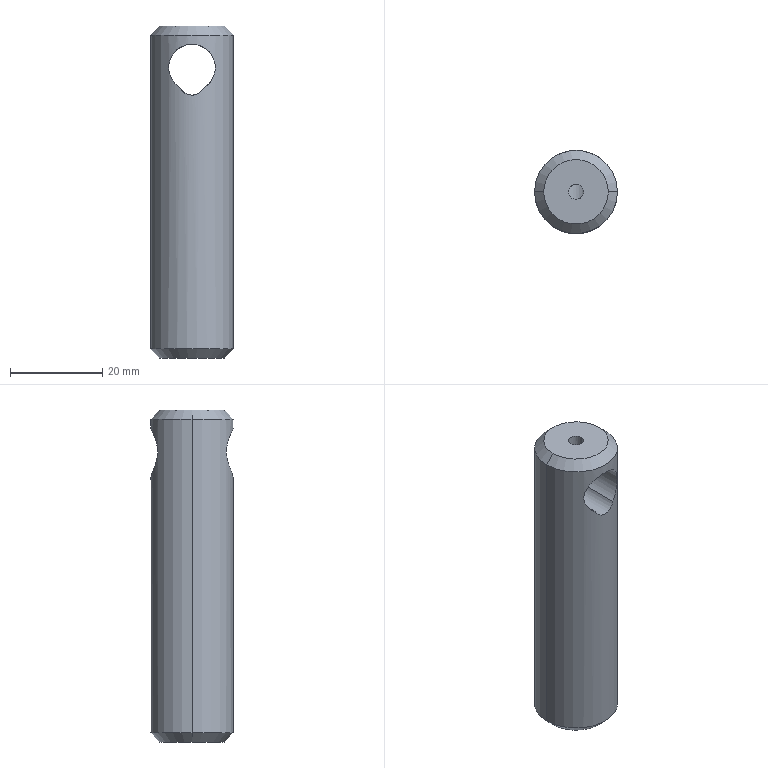Part | SolidWorks | features Chamfer 1, Extrusion 1, HoleWzd 1, ICE 1 | 1 solid | 13 faces | box 18 x 18 x 72 mm | volume 16626 mm3 | cylinder 7 | cone 4 | plane 2 | commonest cylinder face diameters 3.3 x2 10.1 x2 18 x2 6 x1
STEP:
#1=CARTESIAN_POINT('',(7.,0.,72.));
#2=VERTEX_POINT('',#1);
#3=CARTESIAN_POINT('',(-7.,0.,72.));
#4=VERTEX_POINT('',#3);
#5=CARTESIAN_POINT('',(0.,0.,72.));
#6=DIRECTION('',(0.,0.,1.));
#7=DIRECTION('',(1.,0.,0.));
#8=AXIS2_PLACEMENT_3D('',#5,#6,#7);
#9=CIRCLE('',#8,7.);
#10=EDGE_CURVE('',#2,#4,#9,.T.);
#11=ORIENTED_EDGE('',*,*,#10,.F.);
#12=CARTESIAN_POINT('',(9.,0.,70.));
#13=VERTEX_POINT('',#12);
#14=CARTESIAN_POINT('',(7.,0.,72.));
#15=DIRECTION('',(0.7071,0.,-0.7071));
#16=VECTOR('',#15,1000.);
#17=LINE('',#14,#16);
#18=EDGE_CURVE('',#2,#13,#17,.T.);
#19=ORIENTED_EDGE('',*,*,#18,.T.);
#20=CARTESIAN_POINT('',(-9.,0.,70.));
#21=VERTEX_POINT('',#20);
#22=CARTESIAN_POINT('',(0.,0.,70.));
#23=DIRECTION('',(0.,0.,-1.));
#24=DIRECTION('',(1.,0.,0.));
#25=AXIS2_PLACEMENT_3D('',#22,#23,#24);
#26=CIRCLE('',#25,9.);
#27=EDGE_CURVE('',#21,#13,#26,.T.);
#28=ORIENTED_EDGE('',*,*,#27,.F.);
#29=CARTESIAN_POINT('',(-7.,0.,72.));
#30=DIRECTION('',(-0.7071,0.,-0.7071));
#31=VECTOR('',#30,1000.);
#32=LINE('',#29,#31);
#33=EDGE_CURVE('',#4,#21,#32,.T.);
#34=ORIENTED_EDGE('',*,*,#33,.F.);
#35=EDGE_LOOP('',(#11,#19,#28,#34));
#36=FACE_OUTER_BOUND('',#35,.T.);
#37=CARTESIAN_POINT('',(0.,0.,72.));
#38=DIRECTION('',(0.,0.,-1.));
#39=DIRECTION('',(-1.,0.,0.));
#40=AXIS2_PLACEMENT_3D('',#37,#38,#39);
#41=CONICAL_SURFACE('',#40,7.,0.7854);
#42=ADVANCED_FACE('',(#36),#41,.T.);
#43=CARTESIAN_POINT('',(-7.,0.,0.));
#44=VERTEX_POINT('',#43);
#45=CARTESIAN_POINT('',(7.,0.,0.));
#46=VERTEX_POINT('',#45);
#47=CARTESIAN_POINT('',(0.,0.,0.));
#48=DIRECTION('',(0.,0.,-1.));
#49=DIRECTION('',(1.,0.,0.));
#50=AXIS2_PLACEMENT_3D('',#47,#48,#49);
#51=CIRCLE('',#50,7.);
#52=EDGE_CURVE('',#44,#46,#51,.T.);
#53=ORIENTED_EDGE('',*,*,#52,.F.);
#54=CARTESIAN_POINT('',(-9.,0.,2.));
#55=VERTEX_POINT('',#54);
#56=CARTESIAN_POINT('',(-9.,0.,2.));
#57=DIRECTION('',(-0.7071,0.,0.7071));
#58=VECTOR('',#57,1000.);
#59=LINE('',#56,#58);
#60=EDGE_CURVE('',#44,#55,#59,.T.);
#61=ORIENTED_EDGE('',*,*,#60,.T.);
#62=CARTESIAN_POINT('',(9.,0.,2.));
#63=VERTEX_POINT('',#62);
#64=CARTESIAN_POINT('',(0.,0.,2.));
#65=DIRECTION('',(0.,0.,1.));
#66=DIRECTION('',(1.,0.,0.));
#67=AXIS2_PLACEMENT_3D('',#64,#65,#66);
#68=CIRCLE('',#67,9.);
#69=EDGE_CURVE('',#63,#55,#68,.T.);
#70=ORIENTED_EDGE('',*,*,#69,.F.);
#71=CARTESIAN_POINT('',(9.,0.,2.));
#72=DIRECTION('',(0.7071,0.,0.7071));
#73=VECTOR('',#72,1000.);
#74=LINE('',#71,#73);
#75=EDGE_CURVE('',#46,#63,#74,.T.);
#76=ORIENTED_EDGE('',*,*,#75,.F.);
#77=EDGE_LOOP('',(#53,#61,#70,#76));
#78=FACE_OUTER_BOUND('',#77,.T.);
#79=CARTESIAN_POINT('',(0.,0.,2.));
#80=DIRECTION('',(0.,0.,1.));
#81=DIRECTION('',(1.,0.,0.));
#82=AXIS2_PLACEMENT_3D('',#79,#80,#81);
#83=CONICAL_SURFACE('',#82,9.,0.7854);
#84=ADVANCED_FACE('',(#78),#83,.T.);
#85=CARTESIAN_POINT('',(-1.65,0.,67.773));
#86=VERTEX_POINT('',#85);
#87=CARTESIAN_POINT('',(0.,-1.65,68.05));
#88=VERTEX_POINT('',#87);
#89=CARTESIAN_POINT('',(-1.65,0.,67.773));
#90=CARTESIAN_POINT('',(-1.65,-0.2163,67.773));
#91=CARTESIAN_POINT('',(-1.606,-0.4347,67.789));
#92=CARTESIAN_POINT('',(-1.482,-0.7331,67.828));
#93=CARTESIAN_POINT('',(-1.43,-0.8296,67.844));
#94=CARTESIAN_POINT('',(-1.311,-1.008,67.877));
#95=CARTESIAN_POINT('',(-1.243,-1.09,67.895));
#96=CARTESIAN_POINT('',(-1.015,-1.319,67.95));
#97=CARTESIAN_POINT('',(-0.8346,-1.44,67.985));
#98=CARTESIAN_POINT('',(-0.5336,-1.565,68.023));
#99=CARTESIAN_POINT('',(-0.4305,-1.597,68.033));
#100=CARTESIAN_POINT('',(-0.2187,-1.639,68.046));
#101=CARTESIAN_POINT('',(-0.1087,-1.65,68.05));
#102=CARTESIAN_POINT('',(0.,-1.65,68.05));
#103=B_SPLINE_CURVE_WITH_KNOTS('',3,(#89,#90,#91,#92,#93,#94,#95,#96,#97,#98,#99,#100,#101,#102),.UNSPECIFIED.,.F.,.F.,(4,2,2,2,2,2,4),(0.005194,0.005844,0.006168,0.006493,0.007142,0.007466,0.007791),.UNSPECIFIED.);
#104=EDGE_CURVE('',#86,#88,#103,.T.);
#105=ORIENTED_EDGE('',*,*,#104,.F.);
#106=CARTESIAN_POINT('',(-1.65,0.,72.));
#107=VERTEX_POINT('',#106);
#108=CARTESIAN_POINT('',(-1.65,0.,72.));
#109=DIRECTION('',(0.,0.,1.));
#110=VECTOR('',#109,1000.);
#111=LINE('',#108,#110);
#112=EDGE_CURVE('',#86,#107,#111,.T.);
#113=ORIENTED_EDGE('',*,*,#112,.T.);
#114=CARTESIAN_POINT('',(1.65,0.,72.));
#115=VERTEX_POINT('',#114);
#116=CARTESIAN_POINT('',(0.,0.,72.));
#117=DIRECTION('',(0.,0.,1.));
#118=DIRECTION('',(1.,0.,0.));
#119=AXIS2_PLACEMENT_3D('',#116,#117,#118);
#120=CIRCLE('',#119,1.65);
#121=EDGE_CURVE('',#107,#115,#120,.T.);
#122=ORIENTED_EDGE('',*,*,#121,.T.);
#123=CARTESIAN_POINT('',(1.65,0.,67.773));
#124=VERTEX_POINT('',#123);
#125=CARTESIAN_POINT('',(1.65,0.,72.));
#126=DIRECTION('',(0.,0.,1.));
#127=VECTOR('',#126,1000.);
#128=LINE('',#125,#127);
#129=EDGE_CURVE('',#124,#115,#128,.T.);
#130=ORIENTED_EDGE('',*,*,#129,.F.);
#131=CARTESIAN_POINT('',(0.,-1.65,68.05));
#132=CARTESIAN_POINT('',(0.1087,-1.65,68.05));
#133=CARTESIAN_POINT('',(0.2164,-1.639,68.046));
#134=CARTESIAN_POINT('',(0.4295,-1.597,68.033));
#135=CARTESIAN_POINT('',(0.5346,-1.565,68.023));
#136=CARTESIAN_POINT('',(0.8328,-1.441,67.985));
#137=CARTESIAN_POINT('',(1.015,-1.318,67.949));
#138=CARTESIAN_POINT('',(1.242,-1.091,67.895));
#139=CARTESIAN_POINT('',(1.312,-1.007,67.877));
#140=CARTESIAN_POINT('',(1.431,-0.8285,67.843));
#141=CARTESIAN_POINT('',(1.482,-0.7342,67.828));
#142=CARTESIAN_POINT('',(1.565,-0.5349,67.802));
#143=CARTESIAN_POINT('',(1.597,-0.4297,67.791));
#144=CARTESIAN_POINT('',(1.639,-0.2177,67.777));
#145=CARTESIAN_POINT('',(1.65,-0.1098,67.773));
#146=CARTESIAN_POINT('',(1.65,0.,67.773));
#147=B_SPLINE_CURVE_WITH_KNOTS('',3,(#131,#132,#133,#134,#135,#136,#137,#138,#139,#140,#141,#142,#143,#144,#145,#146),.UNSPECIFIED.,.F.,.F.,(4,2,2,2,2,2,2,4),(0.007791,0.008115,0.00844,0.009089,0.009414,0.009738,0.01006,0.01039),.UNSPECIFIED.);
#148=EDGE_CURVE('',#88,#124,#147,.T.);
#149=ORIENTED_EDGE('',*,*,#148,.F.);
#150=EDGE_LOOP('',(#105,#113,#122,#130,#149));
#151=FACE_OUTER_BOUND('',#150,.T.);
#152=CARTESIAN_POINT('',(0.,0.,72.));
#153=DIRECTION('',(0.,0.,1.));
#154=DIRECTION('',(1.,0.,0.));
#155=AXIS2_PLACEMENT_3D('',#152,#153,#154);
#156=CYLINDRICAL_SURFACE('',#155,1.65);
#157=ADVANCED_FACE('',(#151),#156,.F.);
#158=CARTESIAN_POINT('',(0.,-9.,68.05));
#159=VERTEX_POINT('',#158);
#160=CARTESIAN_POINT('',(2.727,-8.577,58.75));
#161=VERTEX_POINT('',#160);
#162=CARTESIAN_POINT('',(0.,-9.,68.05));
#163=CARTESIAN_POINT('',(0.2797,-9.,68.05));
#164=CARTESIAN_POINT('',(0.5548,-8.987,68.027));
#165=CARTESIAN_POINT('',(1.097,-8.937,67.937));
#166=CARTESIAN_POINT('',(1.366,-8.9,67.87));
#167=CARTESIAN_POINT('',(1.885,-8.804,67.693));
#168=CARTESIAN_POINT('',(2.133,-8.747,67.585));
#169=CARTESIAN_POINT('',(2.608,-8.617,67.333));
#170=CARTESIAN_POINT('',(2.836,-8.544,67.187));
#171=CARTESIAN_POINT('',(3.261,-8.391,66.865));
#172=CARTESIAN_POINT('',(3.459,-8.311,66.689));
#173=CARTESIAN_POINT('',(3.825,-8.149,66.308));
#174=CARTESIAN_POINT('',(3.995,-8.066,66.1));
#175=CARTESIAN_POINT('',(4.299,-7.909,65.664));
#176=CARTESIAN_POINT('',(4.432,-7.834,65.435));
#177=CARTESIAN_POINT('',(4.664,-7.698,64.954));
#178=CARTESIAN_POINT('',(4.763,-7.637,64.701));
#179=CARTESIAN_POINT('',(4.919,-7.537,64.175));
#180=CARTESIAN_POINT('',(4.975,-7.5,63.907));
#181=CARTESIAN_POINT('',(5.045,-7.453,63.361));
#182=CARTESIAN_POINT('',(5.057,-7.445,63.079));
#183=CARTESIAN_POINT('',(5.035,-7.46,62.525));
#184=CARTESIAN_POINT('',(5.002,-7.482,62.252));
#185=CARTESIAN_POINT('',(4.891,-7.555,61.713));
#186=CARTESIAN_POINT('',(4.813,-7.606,61.448));
#187=CARTESIAN_POINT('',(4.62,-7.725,60.942));
#188=CARTESIAN_POINT('',(4.504,-7.793,60.7));
#189=CARTESIAN_POINT('',(4.234,-7.943,60.235));
#190=CARTESIAN_POINT('',(4.082,-8.023,60.016));
#191=CARTESIAN_POINT('',(3.582,-8.265,59.401));
#192=CARTESIAN_POINT('',(3.182,-8.432,59.041));
#193=CARTESIAN_POINT('',(2.727,-8.577,58.75));
#194=B_SPLINE_CURVE_WITH_KNOTS('',3,(#162,#163,#164,#165,#166,#167,#168,#169,#170,#171,#172,#173,#174,#175,#176,#177,#178,#179,#180,#181,#182,#183,#184,#185,#186,#187,#188,#189,#190,#191,#192,#193),.UNSPECIFIED.,.F.,.F.,(4,2,2,2,2,2,2,2,2,2,2,2,2,2,2,4),(0.01324,0.01406,0.01489,0.01571,0.01654,0.01736,0.01819,0.01901,0.01984,0.02066,0.02149,0.02231,0.02314,0.02396,0.02479,0.02644),.UNSPECIFIED.);
#195=EDGE_CURVE('',#159,#161,#194,.T.);
#196=ORIENTED_EDGE('',*,*,#195,.F.);
#197=CARTESIAN_POINT('',(0.,-9.,68.05));
#198=DIRECTION('',(0.,1.,0.));
#199=VECTOR('',#198,1000.);
#200=LINE('',#197,#199);
#201=EDGE_CURVE('',#159,#88,#200,.T.);
#202=ORIENTED_EDGE('',*,*,#201,.T.);
#203=ORIENTED_EDGE('',*,*,#148,.T.);
#204=CARTESIAN_POINT('',(0.,1.65,68.05));
#205=VERTEX_POINT('',#204);
#206=CARTESIAN_POINT('',(1.65,0.,67.773));
#207=CARTESIAN_POINT('',(1.65,0.1099,67.773));
#208=CARTESIAN_POINT('',(1.639,0.2177,67.777));
#209=CARTESIAN_POINT('',(1.597,0.4297,67.791));
#210=CARTESIAN_POINT('',(1.565,0.5349,67.802));
#211=CARTESIAN_POINT('',(1.482,0.7344,67.828));
#212=CARTESIAN_POINT('',(1.431,0.8289,67.843));
#213=CARTESIAN_POINT('',(1.311,1.008,67.877));
#214=CARTESIAN_POINT('',(1.242,1.092,67.896));
#215=CARTESIAN_POINT('',(1.015,1.318,67.949));
#216=CARTESIAN_POINT('',(0.8321,1.441,67.985));
#217=CARTESIAN_POINT('',(0.5345,1.565,68.023));
#218=CARTESIAN_POINT('',(0.4296,1.597,68.033));
#219=CARTESIAN_POINT('',(0.2162,1.639,68.047));
#220=CARTESIAN_POINT('',(0.1085,1.65,68.05));
#221=CARTESIAN_POINT('',(0.,1.65,68.05));
#222=B_SPLINE_CURVE_WITH_KNOTS('',3,(#206,#207,#208,#209,#210,#211,#212,#213,#214,#215,#216,#217,#218,#219,#220,#221),.UNSPECIFIED.,.F.,.F.,(4,2,2,2,2,2,2,4),(0.,0.0003247,0.0006495,0.0009742,0.001299,0.001948,0.002273,0.002598),.UNSPECIFIED.);
#223=EDGE_CURVE('',#124,#205,#222,.T.);
#224=ORIENTED_EDGE('',*,*,#223,.T.);
#225=CARTESIAN_POINT('',(0.,9.,68.05));
#226=VERTEX_POINT('',#225);
#227=CARTESIAN_POINT('',(0.,-9.,68.05));
#228=DIRECTION('',(0.,1.,0.));
#229=VECTOR('',#228,1000.);
#230=LINE('',#227,#229);
#231=EDGE_CURVE('',#205,#226,#230,.T.);
#232=ORIENTED_EDGE('',*,*,#231,.T.);
#233=CARTESIAN_POINT('',(2.727,8.577,58.75));
#234=VERTEX_POINT('',#233);
#235=CARTESIAN_POINT('',(2.727,8.577,58.75));
#236=CARTESIAN_POINT('',(3.182,8.432,59.041));
#237=CARTESIAN_POINT('',(3.574,8.268,59.393));
#238=CARTESIAN_POINT('',(4.079,8.025,60.011));
#239=CARTESIAN_POINT('',(4.232,7.944,60.232));
#240=CARTESIAN_POINT('',(4.499,7.796,60.691));
#241=CARTESIAN_POINT('',(4.615,7.728,60.931));
#242=CARTESIAN_POINT('',(4.809,7.608,61.436));
#243=CARTESIAN_POINT('',(4.888,7.557,61.702));
#244=CARTESIAN_POINT('',(5.,7.484,62.24));
#245=CARTESIAN_POINT('',(5.034,7.46,62.513));
#246=CARTESIAN_POINT('',(5.057,7.445,63.07));
#247=CARTESIAN_POINT('',(5.045,7.453,63.35));
#248=CARTESIAN_POINT('',(4.977,7.499,63.897));
#249=CARTESIAN_POINT('',(4.921,7.536,64.167));
#250=CARTESIAN_POINT('',(4.765,7.636,64.695));
#251=CARTESIAN_POINT('',(4.667,7.696,64.947));
#252=CARTESIAN_POINT('',(4.434,7.833,65.432));
#253=CARTESIAN_POINT('',(4.298,7.909,65.665));
#254=CARTESIAN_POINT('',(3.993,8.067,66.103));
#255=CARTESIAN_POINT('',(3.826,8.149,66.307));
#256=CARTESIAN_POINT('',(3.459,8.311,66.689));
#257=CARTESIAN_POINT('',(3.258,8.393,66.868));
#258=CARTESIAN_POINT('',(2.832,8.546,67.19));
#259=CARTESIAN_POINT('',(2.607,8.618,67.333));
#260=CARTESIAN_POINT('',(2.134,8.747,67.585));
#261=CARTESIAN_POINT('',(1.884,8.805,67.694));
#262=CARTESIAN_POINT('',(1.102,8.948,67.959));
#263=CARTESIAN_POINT('',(0.5607,9.,68.05));
#264=CARTESIAN_POINT('',(0.,9.,68.05));
#265=B_SPLINE_CURVE_WITH_KNOTS('',3,(#235,#236,#237,#238,#239,#240,#241,#242,#243,#244,#245,#246,#247,#248,#249,#250,#251,#252,#253,#254,#255,#256,#257,#258,#259,#260,#261,#262,#263,#264),.UNSPECIFIED.,.F.,.F.,(4,2,2,2,2,2,2,2,2,2,2,2,2,2,4),(0.,0.001654,0.002482,0.003309,0.004136,0.004963,0.005791,0.006618,0.007445,0.008272,0.0091,0.009927,0.01075,0.01158,0.01324),.UNSPECIFIED.);
#266=EDGE_CURVE('',#234,#226,#265,.T.);
#267=ORIENTED_EDGE('',*,*,#266,.F.);
#268=CARTESIAN_POINT('',(2.727,-9.,58.75));
#269=DIRECTION('',(0.,1.,0.));
#270=VECTOR('',#269,1000.);
#271=LINE('',#268,#270);
#272=EDGE_CURVE('',#161,#234,#271,.T.);
#273=ORIENTED_EDGE('',*,*,#272,.F.);
#274=EDGE_LOOP('',(#196,#202,#203,#224,#232,#267,#273));
#275=FACE_OUTER_BOUND('',#274,.T.);
#276=CARTESIAN_POINT('',(0.,-9.,63.));
#277=DIRECTION('',(0.,1.,0.));
#278=DIRECTION('',(0.,0.,1.));
#279=AXIS2_PLACEMENT_3D('',#276,#277,#278);
#280=CYLINDRICAL_SURFACE('',#279,5.05);
#281=ADVANCED_FACE('',(#275),#280,.F.);
#282=CARTESIAN_POINT('',(-2.727,8.577,58.75));
#283=VERTEX_POINT('',#282);
#284=CARTESIAN_POINT('',(-2.727,8.577,58.75));
#285=CARTESIAN_POINT('',(-2.607,8.615,58.488));
#286=CARTESIAN_POINT('',(-2.454,8.661,58.251));
#287=CARTESIAN_POINT('',(-2.175,8.734,57.929));
#288=CARTESIAN_POINT('',(-2.073,8.759,57.827));
#289=CARTESIAN_POINT('',(-1.859,8.807,57.641));
#290=CARTESIAN_POINT('',(-1.746,8.83,57.557));
#291=CARTESIAN_POINT('',(-1.389,8.895,57.326));
#292=CARTESIAN_POINT('',(-1.125,8.934,57.204));
#293=CARTESIAN_POINT('',(-0.5789,8.986,57.043));
#294=CARTESIAN_POINT('',(-0.2884,9.,57.));
#295=CARTESIAN_POINT('',(0.1414,9.,57.));
#296=CARTESIAN_POINT('',(0.2842,8.997,57.01));
#297=CARTESIAN_POINT('',(0.5687,8.983,57.051));
#298=CARTESIAN_POINT('',(0.7111,8.973,57.082));
#299=CARTESIAN_POINT('',(0.9859,8.947,57.163));
#300=CARTESIAN_POINT('',(1.119,8.931,57.213));
#301=CARTESIAN_POINT('',(1.378,8.895,57.332));
#302=CARTESIAN_POINT('',(1.505,8.874,57.401));
#303=CARTESIAN_POINT('',(1.864,8.808,57.632));
#304=CARTESIAN_POINT('',(2.078,8.759,57.817));
#305=CARTESIAN_POINT('',(2.453,8.661,58.25));
#306=CARTESIAN_POINT('',(2.607,8.615,58.488));
#307=CARTESIAN_POINT('',(2.727,8.577,58.75));
#308=B_SPLINE_CURVE_WITH_KNOTS('',3,(#284,#285,#286,#287,#288,#289,#290,#291,#292,#293,#294,#295,#296,#297,#298,#299,#300,#301,#302,#303,#304,#305,#306,#307),.UNSPECIFIED.,.F.,.F.,(4,2,2,2,2,2,2,2,2,2,2,4),(0.,0.0008586,0.001288,0.001717,0.002576,0.003434,0.003864,0.004293,0.004722,0.005152,0.00601,0.006869),.UNSPECIFIED.);
#309=EDGE_CURVE('',#283,#234,#308,.T.);
#310=ORIENTED_EDGE('',*,*,#309,.T.);
#311=ORIENTED_EDGE('',*,*,#266,.T.);
#312=CARTESIAN_POINT('',(0.,9.,68.05));
#313=CARTESIAN_POINT('',(-0.2797,9.,68.05));
#314=CARTESIAN_POINT('',(-0.5548,8.987,68.027));
#315=CARTESIAN_POINT('',(-1.097,8.937,67.937));
#316=CARTESIAN_POINT('',(-1.366,8.9,67.87));
#317=CARTESIAN_POINT('',(-1.885,8.804,67.693));
#318=CARTESIAN_POINT('',(-2.133,8.747,67.585));
#319=CARTESIAN_POINT('',(-2.608,8.617,67.333));
#320=CARTESIAN_POINT('',(-2.836,8.544,67.187));
#321=CARTESIAN_POINT('',(-3.261,8.391,66.865));
#322=CARTESIAN_POINT('',(-3.459,8.311,66.689));
#323=CARTESIAN_POINT('',(-3.825,8.149,66.308));
#324=CARTESIAN_POINT('',(-3.995,8.066,66.1));
#325=CARTESIAN_POINT('',(-4.299,7.909,65.664));
#326=CARTESIAN_POINT('',(-4.432,7.834,65.435));
#327=CARTESIAN_POINT('',(-4.664,7.698,64.954));
#328=CARTESIAN_POINT('',(-4.763,7.637,64.701));
#329=CARTESIAN_POINT('',(-4.919,7.537,64.175));
#330=CARTESIAN_POINT('',(-4.975,7.5,63.907));
#331=CARTESIAN_POINT('',(-5.045,7.453,63.361));
#332=CARTESIAN_POINT('',(-5.057,7.445,63.079));
#333=CARTESIAN_POINT('',(-5.035,7.46,62.525));
#334=CARTESIAN_POINT('',(-5.002,7.482,62.252));
#335=CARTESIAN_POINT('',(-4.891,7.555,61.713));
#336=CARTESIAN_POINT('',(-4.813,7.606,61.448));
#337=CARTESIAN_POINT('',(-4.62,7.725,60.942));
#338=CARTESIAN_POINT('',(-4.504,7.793,60.7));
#339=CARTESIAN_POINT('',(-4.234,7.943,60.235));
#340=CARTESIAN_POINT('',(-4.082,8.023,60.016));
#341=CARTESIAN_POINT('',(-3.582,8.265,59.401));
#342=CARTESIAN_POINT('',(-3.182,8.432,59.041));
#343=CARTESIAN_POINT('',(-2.727,8.577,58.75));
#344=B_SPLINE_CURVE_WITH_KNOTS('',3,(#312,#313,#314,#315,#316,#317,#318,#319,#320,#321,#322,#323,#324,#325,#326,#327,#328,#329,#330,#331,#332,#333,#334,#335,#336,#337,#338,#339,#340,#341,#342,#343),.UNSPECIFIED.,.F.,.F.,(4,2,2,2,2,2,2,2,2,2,2,2,2,2,2,4),(0.01324,0.01406,0.01489,0.01571,0.01654,0.01736,0.01819,0.01901,0.01984,0.02066,0.02149,0.02231,0.02314,0.02396,0.02479,0.02644),.UNSPECIFIED.);
#345=EDGE_CURVE('',#226,#283,#344,.T.);
#346=ORIENTED_EDGE('',*,*,#345,.T.);
#347=EDGE_LOOP('',(#310,#311,#346));
#348=FACE_BOUND('',#347,.T.);
#349=ORIENTED_EDGE('',*,*,#27,.T.);
#350=CARTESIAN_POINT('',(9.,0.,72.));
#351=DIRECTION('',(0.,0.,-1.));
#352=VECTOR('',#351,1000.);
#353=LINE('',#350,#352);
#354=EDGE_CURVE('',#13,#63,#353,.T.);
#355=ORIENTED_EDGE('',*,*,#354,.T.);
#356=ORIENTED_EDGE('',*,*,#69,.T.);
#357=CARTESIAN_POINT('',(-9.,0.,72.));
#358=DIRECTION('',(0.,0.,-1.));
#359=VECTOR('',#358,1000.);
#360=LINE('',#357,#359);
#361=EDGE_CURVE('',#21,#55,#360,.T.);
#362=ORIENTED_EDGE('',*,*,#361,.F.);
#363=EDGE_LOOP('',(#349,#355,#356,#362));
#364=FACE_OUTER_BOUND('',#363,.T.);
#365=CARTESIAN_POINT('',(0.,0.,72.));
#366=DIRECTION('',(0.,0.,-1.));
#367=DIRECTION('',(-1.,0.,0.));
#368=AXIS2_PLACEMENT_3D('',#365,#366,#367);
#369=CYLINDRICAL_SURFACE('',#368,9.);
#370=ADVANCED_FACE('',(#348,#364),#369,.T.);
#371=ORIENTED_EDGE('',*,*,#354,.F.);
#372=CARTESIAN_POINT('',(0.,0.,70.));
#373=DIRECTION('',(0.,0.,-1.));
#374=DIRECTION('',(1.,0.,0.));
#375=AXIS2_PLACEMENT_3D('',#372,#373,#374);
#376=CIRCLE('',#375,9.);
#377=EDGE_CURVE('',#13,#21,#376,.T.);
#378=ORIENTED_EDGE('',*,*,#377,.T.);
#379=ORIENTED_EDGE('',*,*,#361,.T.);
#380=CARTESIAN_POINT('',(0.,0.,2.));
#381=DIRECTION('',(0.,0.,1.));
#382=DIRECTION('',(1.,0.,0.));
#383=AXIS2_PLACEMENT_3D('',#380,#381,#382);
#384=CIRCLE('',#383,9.);
#385=EDGE_CURVE('',#55,#63,#384,.T.);
#386=ORIENTED_EDGE('',*,*,#385,.T.);
#387=EDGE_LOOP('',(#371,#378,#379,#386));
#388=FACE_OUTER_BOUND('',#387,.T.);
#389=CARTESIAN_POINT('',(-2.727,-8.577,58.75));
#390=VERTEX_POINT('',#389);
#391=CARTESIAN_POINT('',(2.727,-8.577,58.75));
#392=CARTESIAN_POINT('',(2.607,-8.615,58.488));
#393=CARTESIAN_POINT('',(2.454,-8.661,58.251));
#394=CARTESIAN_POINT('',(2.175,-8.734,57.929));
#395=CARTESIAN_POINT('',(2.073,-8.759,57.827));
#396=CARTESIAN_POINT('',(1.859,-8.807,57.641));
#397=CARTESIAN_POINT('',(1.746,-8.83,57.557));
#398=CARTESIAN_POINT('',(1.389,-8.895,57.326));
#399=CARTESIAN_POINT('',(1.125,-8.934,57.204));
#400=CARTESIAN_POINT('',(0.5789,-8.986,57.043));
#401=CARTESIAN_POINT('',(0.2884,-9.,57.));
#402=CARTESIAN_POINT('',(-0.1414,-9.,57.));
#403=CARTESIAN_POINT('',(-0.2842,-8.997,57.01));
#404=CARTESIAN_POINT('',(-0.5687,-8.983,57.051));
#405=CARTESIAN_POINT('',(-0.7111,-8.973,57.082));
#406=CARTESIAN_POINT('',(-0.9859,-8.947,57.163));
#407=CARTESIAN_POINT('',(-1.119,-8.931,57.213));
#408=CARTESIAN_POINT('',(-1.378,-8.895,57.332));
#409=CARTESIAN_POINT('',(-1.505,-8.874,57.401));
#410=CARTESIAN_POINT('',(-1.864,-8.808,57.632));
#411=CARTESIAN_POINT('',(-2.078,-8.759,57.817));
#412=CARTESIAN_POINT('',(-2.453,-8.661,58.25));
#413=CARTESIAN_POINT('',(-2.607,-8.615,58.488));
#414=CARTESIAN_POINT('',(-2.727,-8.577,58.75));
#415=B_SPLINE_CURVE_WITH_KNOTS('',3,(#391,#392,#393,#394,#395,#396,#397,#398,#399,#400,#401,#402,#403,#404,#405,#406,#407,#408,#409,#410,#411,#412,#413,#414),.UNSPECIFIED.,.F.,.F.,(4,2,2,2,2,2,2,2,2,2,2,4),(0.,0.0008586,0.001288,0.001717,0.002576,0.003434,0.003864,0.004293,0.004722,0.005152,0.00601,0.006869),.UNSPECIFIED.);
#416=EDGE_CURVE('',#161,#390,#415,.T.);
#417=ORIENTED_EDGE('',*,*,#416,.T.);
#418=CARTESIAN_POINT('',(-2.727,-8.577,58.75));
#419=CARTESIAN_POINT('',(-3.182,-8.432,59.041));
#420=CARTESIAN_POINT('',(-3.574,-8.268,59.393));
#421=CARTESIAN_POINT('',(-4.079,-8.025,60.011));
#422=CARTESIAN_POINT('',(-4.232,-7.944,60.232));
#423=CARTESIAN_POINT('',(-4.499,-7.796,60.691));
#424=CARTESIAN_POINT('',(-4.615,-7.728,60.931));
#425=CARTESIAN_POINT('',(-4.809,-7.608,61.436));
#426=CARTESIAN_POINT('',(-4.888,-7.557,61.702));
#427=CARTESIAN_POINT('',(-5.,-7.484,62.24));
#428=CARTESIAN_POINT('',(-5.034,-7.46,62.513));
#429=CARTESIAN_POINT('',(-5.057,-7.445,63.07));
#430=CARTESIAN_POINT('',(-5.045,-7.453,63.35));
#431=CARTESIAN_POINT('',(-4.977,-7.499,63.897));
#432=CARTESIAN_POINT('',(-4.921,-7.536,64.167));
#433=CARTESIAN_POINT('',(-4.765,-7.636,64.695));
#434=CARTESIAN_POINT('',(-4.667,-7.696,64.947));
#435=CARTESIAN_POINT('',(-4.434,-7.833,65.432));
#436=CARTESIAN_POINT('',(-4.298,-7.909,65.665));
#437=CARTESIAN_POINT('',(-3.993,-8.067,66.103));
#438=CARTESIAN_POINT('',(-3.826,-8.149,66.307));
#439=CARTESIAN_POINT('',(-3.459,-8.311,66.689));
#440=CARTESIAN_POINT('',(-3.258,-8.393,66.868));
#441=CARTESIAN_POINT('',(-2.832,-8.546,67.19));
#442=CARTESIAN_POINT('',(-2.607,-8.618,67.333));
#443=CARTESIAN_POINT('',(-2.134,-8.747,67.585));
#444=CARTESIAN_POINT('',(-1.884,-8.805,67.694));
#445=CARTESIAN_POINT('',(-1.102,-8.948,67.959));
#446=CARTESIAN_POINT('',(-0.5607,-9.,68.05));
#447=CARTESIAN_POINT('',(0.,-9.,68.05));
#448=B_SPLINE_CURVE_WITH_KNOTS('',3,(#418,#419,#420,#421,#422,#423,#424,#425,#426,#427,#428,#429,#430,#431,#432,#433,#434,#435,#436,#437,#438,#439,#440,#441,#442,#443,#444,#445,#446,#447),.UNSPECIFIED.,.F.,.F.,(4,2,2,2,2,2,2,2,2,2,2,2,2,2,4),(0.,0.001654,0.002482,0.003309,0.004136,0.004963,0.005791,0.006618,0.007445,0.008272,0.0091,0.009927,0.01075,0.01158,0.01324),.UNSPECIFIED.);
#449=EDGE_CURVE('',#390,#159,#448,.T.);
#450=ORIENTED_EDGE('',*,*,#449,.T.);
#451=ORIENTED_EDGE('',*,*,#195,.T.);
#452=EDGE_LOOP('',(#417,#450,#451));
#453=FACE_BOUND('',#452,.T.);
#454=CARTESIAN_POINT('',(0.,0.,72.));
#455=DIRECTION('',(0.,0.,-1.));
#456=DIRECTION('',(-1.,0.,0.));
#457=AXIS2_PLACEMENT_3D('',#454,#455,#456);
#458=CYLINDRICAL_SURFACE('',#457,9.);
#459=ADVANCED_FACE('',(#388,#453),#458,.T.);
#460=CARTESIAN_POINT('',(0.,0.,72.));
#461=DIRECTION('',(0.,0.,1.));
#462=DIRECTION('',(1.,0.,0.));
#463=AXIS2_PLACEMENT_3D('',#460,#461,#462);
#464=CIRCLE('',#463,7.);
#465=EDGE_CURVE('',#4,#2,#464,.T.);
#466=ORIENTED_EDGE('',*,*,#465,.T.);
#467=ORIENTED_EDGE('',*,*,#10,.T.);
#468=EDGE_LOOP('',(#466,#467));
#469=FACE_OUTER_BOUND('',#468,.T.);
#470=CARTESIAN_POINT('',(0.,0.,72.));
#471=DIRECTION('',(0.,0.,1.));
#472=DIRECTION('',(1.,0.,0.));
#473=AXIS2_PLACEMENT_3D('',#470,#471,#472);
#474=CIRCLE('',#473,1.65);
#475=EDGE_CURVE('',#115,#107,#474,.T.);
#476=ORIENTED_EDGE('',*,*,#475,.F.);
#477=ORIENTED_EDGE('',*,*,#121,.F.);
#478=EDGE_LOOP('',(#476,#477));
#479=FACE_BOUND('',#478,.T.);
#480=CARTESIAN_POINT('',(0.,0.,72.));
#481=DIRECTION('',(0.,0.,1.));
#482=DIRECTION('',(1.,0.,0.));
#483=AXIS2_PLACEMENT_3D('',#480,#481,#482);
#484=PLANE('',#483);
#485=ADVANCED_FACE('',(#469,#479),#484,.T.);
#486=CARTESIAN_POINT('',(0.,0.,0.));
#487=DIRECTION('',(0.,0.,-1.));
#488=DIRECTION('',(1.,0.,0.));
#489=AXIS2_PLACEMENT_3D('',#486,#487,#488);
#490=CIRCLE('',#489,7.);
#491=EDGE_CURVE('',#46,#44,#490,.T.);
#492=ORIENTED_EDGE('',*,*,#491,.T.);
#493=ORIENTED_EDGE('',*,*,#52,.T.);
#494=EDGE_LOOP('',(#492,#493));
#495=FACE_OUTER_BOUND('',#494,.T.);
#496=CARTESIAN_POINT('',(0.,0.,0.));
#497=DIRECTION('',(0.,0.,1.));
#498=DIRECTION('',(1.,0.,0.));
#499=AXIS2_PLACEMENT_3D('',#496,#497,#498);
#500=PLANE('',#499);
#501=ADVANCED_FACE('',(#495),#500,.F.);
#502=CARTESIAN_POINT('',(-2.727,-9.,58.75));
#503=DIRECTION('',(0.,1.,0.));
#504=VECTOR('',#503,1000.);
#505=LINE('',#502,#504);
#506=EDGE_CURVE('',#390,#283,#505,.T.);
#507=ORIENTED_EDGE('',*,*,#506,.F.);
#508=ORIENTED_EDGE('',*,*,#416,.F.);
#509=ORIENTED_EDGE('',*,*,#272,.T.);
#510=ORIENTED_EDGE('',*,*,#309,.F.);
#511=EDGE_LOOP('',(#507,#508,#509,#510));
#512=FACE_OUTER_BOUND('',#511,.T.);
#513=CARTESIAN_POINT('',(0.,-9.,60.));
#514=DIRECTION('',(0.,1.,0.));
#515=DIRECTION('',(0.,0.,1.));
#516=AXIS2_PLACEMENT_3D('',#513,#514,#515);
#517=CYLINDRICAL_SURFACE('',#516,3.);
#518=ADVANCED_FACE('',(#512),#517,.F.);
#519=ORIENTED_EDGE('',*,*,#201,.F.);
#520=ORIENTED_EDGE('',*,*,#449,.F.);
#521=ORIENTED_EDGE('',*,*,#506,.T.);
#522=ORIENTED_EDGE('',*,*,#345,.F.);
#523=ORIENTED_EDGE('',*,*,#231,.F.);
#524=CARTESIAN_POINT('',(0.,1.65,68.05));
#525=CARTESIAN_POINT('',(-0.1085,1.65,68.05));
#526=CARTESIAN_POINT('',(-0.2186,1.639,68.046));
#527=CARTESIAN_POINT('',(-0.4308,1.596,68.033));
#528=CARTESIAN_POINT('',(-0.5341,1.565,68.023));
#529=CARTESIAN_POINT('',(-0.8352,1.44,67.985));
#530=CARTESIAN_POINT('',(-1.016,1.318,67.949));
#531=CARTESIAN_POINT('',(-1.244,1.09,67.895));
#532=CARTESIAN_POINT('',(-1.311,1.007,67.877));
#533=CARTESIAN_POINT('',(-1.431,0.829,67.844));
#534=CARTESIAN_POINT('',(-1.482,0.7325,67.828));
#535=CARTESIAN_POINT('',(-1.565,0.5339,67.802));
#536=CARTESIAN_POINT('',(-1.596,0.431,67.791));
#537=CARTESIAN_POINT('',(-1.639,0.2176,67.777));
#538=CARTESIAN_POINT('',(-1.65,0.1082,67.773));
#539=CARTESIAN_POINT('',(-1.65,0.,67.773));
#540=B_SPLINE_CURVE_WITH_KNOTS('',3,(#524,#525,#526,#527,#528,#529,#530,#531,#532,#533,#534,#535,#536,#537,#538,#539),.UNSPECIFIED.,.F.,.F.,(4,2,2,2,2,2,2,4),(0.002598,0.002923,0.003247,0.003896,0.004221,0.004545,0.00487,0.005194),.UNSPECIFIED.);
#541=EDGE_CURVE('',#205,#86,#540,.T.);
#542=ORIENTED_EDGE('',*,*,#541,.T.);
#543=ORIENTED_EDGE('',*,*,#104,.T.);
#544=EDGE_LOOP('',(#519,#520,#521,#522,#523,#542,#543));
#545=FACE_OUTER_BOUND('',#544,.T.);
#546=CARTESIAN_POINT('',(0.,-9.,63.));
#547=DIRECTION('',(0.,1.,0.));
#548=DIRECTION('',(0.,0.,1.));
#549=AXIS2_PLACEMENT_3D('',#546,#547,#548);
#550=CYLINDRICAL_SURFACE('',#549,5.05);
#551=ADVANCED_FACE('',(#545),#550,.F.);
#552=ORIENTED_EDGE('',*,*,#112,.F.);
#553=ORIENTED_EDGE('',*,*,#541,.F.);
#554=ORIENTED_EDGE('',*,*,#223,.F.);
#555=ORIENTED_EDGE('',*,*,#129,.T.);
#556=ORIENTED_EDGE('',*,*,#475,.T.);
#557=EDGE_LOOP('',(#552,#553,#554,#555,#556));
#558=FACE_OUTER_BOUND('',#557,.T.);
#559=CARTESIAN_POINT('',(0.,0.,72.));
#560=DIRECTION('',(0.,0.,1.));
#561=DIRECTION('',(1.,0.,0.));
#562=AXIS2_PLACEMENT_3D('',#559,#560,#561);
#563=CYLINDRICAL_SURFACE('',#562,1.65);
#564=ADVANCED_FACE('',(#558),#563,.F.);
#565=ORIENTED_EDGE('',*,*,#60,.F.);
#566=ORIENTED_EDGE('',*,*,#491,.F.);
#567=ORIENTED_EDGE('',*,*,#75,.T.);
#568=ORIENTED_EDGE('',*,*,#385,.F.);
#569=EDGE_LOOP('',(#565,#566,#567,#568));
#570=FACE_OUTER_BOUND('',#569,.T.);
#571=CARTESIAN_POINT('',(0.,0.,2.));
#572=DIRECTION('',(0.,0.,1.));
#573=DIRECTION('',(1.,0.,0.));
#574=AXIS2_PLACEMENT_3D('',#571,#572,#573);
#575=CONICAL_SURFACE('',#574,9.,0.7854);
#576=ADVANCED_FACE('',(#570),#575,.T.);
#577=ORIENTED_EDGE('',*,*,#18,.F.);
#578=ORIENTED_EDGE('',*,*,#465,.F.);
#579=ORIENTED_EDGE('',*,*,#33,.T.);
#580=ORIENTED_EDGE('',*,*,#377,.F.);
#581=EDGE_LOOP('',(#577,#578,#579,#580));
#582=FACE_OUTER_BOUND('',#581,.T.);
#583=CARTESIAN_POINT('',(0.,0.,72.));
#584=DIRECTION('',(0.,0.,-1.));
#585=DIRECTION('',(-1.,0.,0.));
#586=AXIS2_PLACEMENT_3D('',#583,#584,#585);
#587=CONICAL_SURFACE('',#586,7.,0.7854);
#588=ADVANCED_FACE('',(#582),#587,.T.);
#589=CLOSED_SHELL('',(#42,#84,#157,#281,#370,#459,#485,#501,#518,#551,#564,#576,#588));
#590=MANIFOLD_SOLID_BREP('',#589);
#591=CARTESIAN_POINT('',(0.,0.,0.));
#592=DIRECTION('',(0.,0.,1.));
#593=DIRECTION('',(1.,0.,0.));
#594=AXIS2_PLACEMENT_3D('',#591,#592,#593);
#595=(LENGTH_UNIT()NAMED_UNIT(*)SI_UNIT(.MILLI.,.METRE.));
#596=UNCERTAINTY_MEASURE_WITH_UNIT(LENGTH_MEASURE(0.00001),#595,'','');
#597=(NAMED_UNIT(*)PLANE_ANGLE_UNIT()SI_UNIT($,.RADIAN.));
#598=(NAMED_UNIT(*)SI_UNIT($,.STERADIAN.)SOLID_ANGLE_UNIT());
#599=(GEOMETRIC_REPRESENTATION_CONTEXT(3)GLOBAL_UNCERTAINTY_ASSIGNED_CONTEXT((#596))GLOBAL_UNIT_ASSIGNED_CONTEXT((#595,#597,#598))REPRESENTATION_CONTEXT('',''));
#600=ADVANCED_BREP_SHAPE_REPRESENTATION('',(#590,#594),#599);